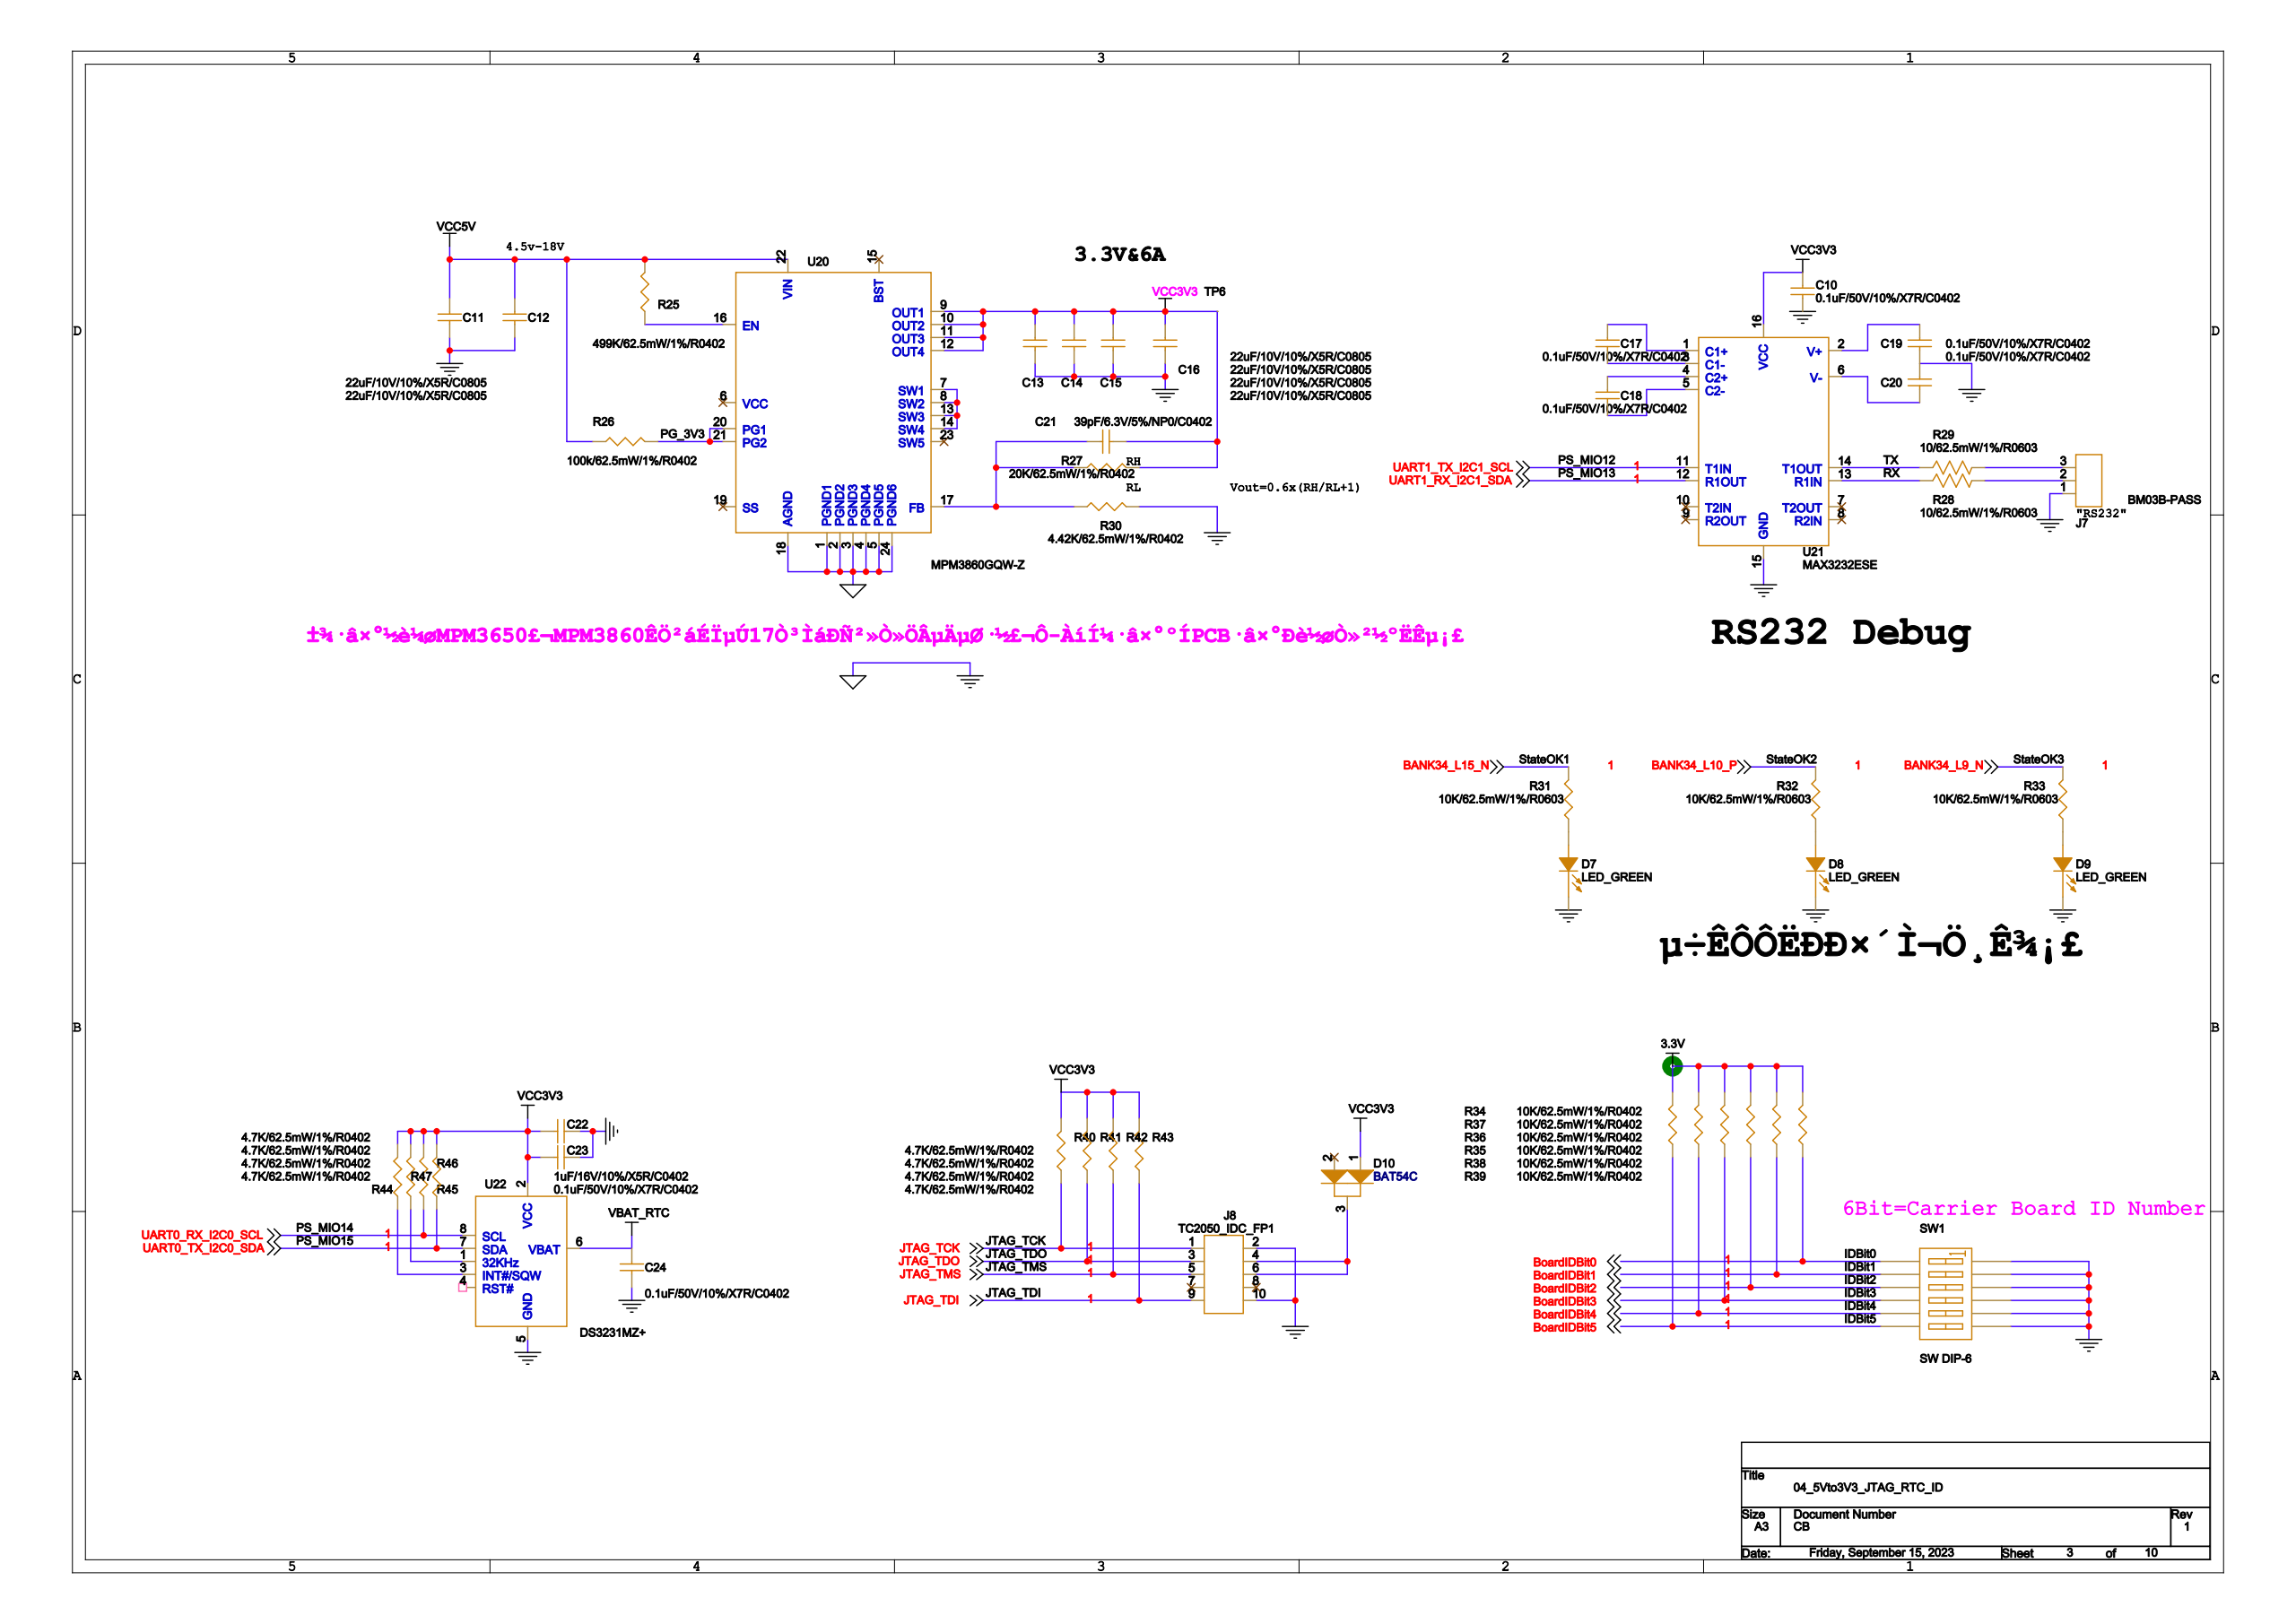Circuit board | Cadence Allegro | 634 parts | 645 nets | one sheet of the schematic
Parts on this sheet (reference | value | footprint):
C10 | 0.1uF/50V/10%/X7R/C0402 | 0402
C11 | 22uF/10V/10%/X5R/C0805 | 0805
C12 | 22uF/10V/10%/X5R/C0805 | 0805
C13 | 22uF/10V/10%/X5R/C0805 | 0805
C14 | 22uF/10V/10%/X5R/C0805 | 0805
C15 | 22uF/10V/10%/X5R/C0805 | 0805
C16 | 22uF/10V/10%/X5R/C0805 | 0805
C17 | 0.1uF/50V/10%/X7R/C0402 | 0402
C18 | 0.1uF/50V/10%/X7R/C0402 | 0402
C19 | 0.1uF/50V/10%/X7R/C0402 | 0402
C20 | 0.1uF/50V/10%/X7R/C0402 | 0402
C21 | 39pF/6.3V/5%/NP0/C0402 | 0402
C22 | 1uF/16V/10%/X5R/C0402 | 0402
C23 | 0.1uF/50V/10%/X7R/C0402 | 0402
C24 | 0.1uF/50V/10%/X7R/C0402 | 0402
D7 | LED_GREEN | LED0805
D8 | LED_GREEN | LED0805
D9 | LED_GREEN | LED0805
D10 | BAT54C | SOT23
J7 | BM03B-PASS | BM03B-PASS
J8 | TC2050_IDC_FP1 | JTAG-10
R25 | 499K/62.5mW/1%/R0402 | 0402
R26 | 100k/62.5mW/1%/R0402 | 0402
R27 | 20K/62.5mW/1%/R0402 | 0402
R28 | 10/62.5mW/1%/R0603 | 0603R
R29 | 10/62.5mW/1%/R0603 | 0603R
R30 | 4.42K/62.5mW/1%/R0402 | 0402
R31 | 10K/62.5mW/1%/R0603 | 0603R
R32 | 10K/62.5mW/1%/R0603 | 0603R
R33 | 10K/62.5mW/1%/R0603 | 0603R
R34 | 10K/62.5mW/1%/R0402 | 0402
R35 | 10K/62.5mW/1%/R0402 | 0402
R36 | 10K/62.5mW/1%/R0402 | 0402
R37 | 10K/62.5mW/1%/R0402 | 0402
R38 | 10K/62.5mW/1%/R0402 | 0402
R39 | 10K/62.5mW/1%/R0402 | 0402
R40 | 4.7K/62.5mW/1%/R0402 | 0402
R41 | 4.7K/62.5mW/1%/R0402 | 0402
R42 | 4.7K/62.5mW/1%/R0402 | 0402
R43 | 4.7K/62.5mW/1%/R0402 | 0402
R44 | 4.7K/62.5mW/1%/R0402 | 0402
R45 | 4.7K/62.5mW/1%/R0402 | 0402
R46 | 4.7K/62.5mW/1%/R0402 | 0402
R47 | 4.7K/62.5mW/1%/R0402 | 0402
SW1 | SW DIP-6 | W-SMD_12P-L9_3-W5_4-P1_27-LS2
TP6 | TEST POINT A | TEST_12MM
U20 | MPM3860GQW-Z | MPM3650GQW
U21 | MAX3232ESE | SO16
U22 | DS3231MZ+ | SO8
Nets of these parts (net: part-pin ...):
AGND: C10-2 C11-2 C12-2 C13-2 C14-2 C15-2 C16-2 C19-2 C20-1 C22-1 C23-1 C24-2 D7-2 D8-2 D9-2 J7-1 J8-2 J8-10 R30-1 SW1-7 SW1-8 SW1-9 SW1-10 SW1-11 SW1-12 U20-1 U20-2 U20-3 U20-4 U20-5 U20-18 U20-24 U21-15 U22-5
3.3V: C10-1 C13-1 C14-1 C15-1 C16-1 C21-2 C22-2 C23-2 D10-1 R27-1 R34-1 R35-1 R36-1 R37-1 R38-1 R39-1 R40-1 R41-1 R42-1 R43-1 R44-1 R45-1 R46-1 R47-1 TP6-1 U20-9 U20-10 U20-11 U20-12 U21-16 U22-2
BOARDIDBIT5: R34-2 SW1-6
BOARDIDBIT4: R35-2 SW1-5
BANK34_L9_N: R33-2
BOARDIDBIT3: R36-2 SW1-4
BANK34_L10_P: R32-2
BOARDIDBIT2: R37-2 SW1-3
BANK34_L15_N: R31-2
BOARDIDBIT1: R38-2 SW1-2
BOARDIDBIT0: R39-2 SW1-1
VCC5V: C11-1 C12-1 R25-1 R26-2 U20-22
JTAG_TDO: J8-3 R41-2
JTAG_TMS: J8-5 R42-2
JTAG_TDI: J8-9 R43-2
JTAG_TCK: J8-1 R40-2
UART0_RX_I2C0_SCL: R46-2 U22-8
UART0_TX_I2C0_SDA: R47-2 U22-7
UART1_TX_I2C1_SCL: U21-11
UART1_RX_I2C1_SDA: U21-12
N23857910: D10-3 J8-4 J8-6
N23931017: J7-2 R28-2
N23931015: J7-3 R29-2
N23930865: C17-1 U21-1
N23930898: C17-2 U21-3
N23930926: C18-1 U21-4
N23930940: C18-2 U21-5
RX: R28-1 U21-13
TX: R29-1 U21-14
N23930874: C19-1 U21-2
N23930928: C20-2 U21-6
N239315640: D7-1 R31-1
N239315840: D8-1 R32-1
N239316020: D9-1 R33-1
VBAT_RTC: C24-1 U22-6
N23155169: C21-1 R27-2 R30-2 U20-17
N23155064: R25-2 U20-16
PG_3V3: R26-1 U20-20 U20-21
N23857516: R44-2 U22-3
N23857518: R45-2 U22-1
N23155134: U20-7 U20-8 U20-13 U20-14